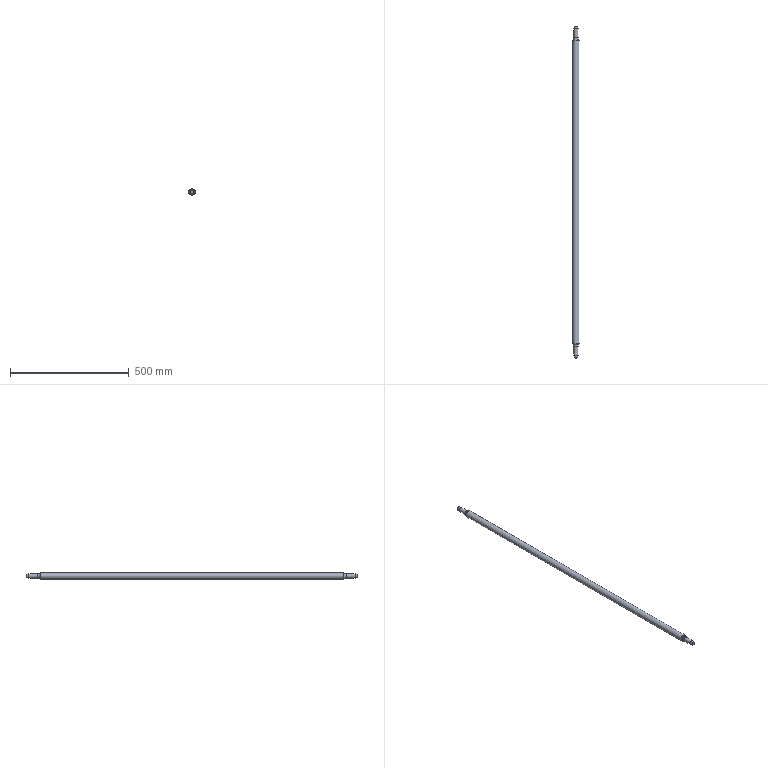Part | NX | features CHAMFER 4, DATUM_CSYS 3, SKETCH 2, Container 1, EXTRACT_BODY 1, EXTRUDE 1, FACE_BLEND 1, Geometry Instance 1, SUBTRACT 1, SWP104 1, SYMBOLIC_THREAD 1 | 1 solid | 31 faces | box 28 x 1395 x 28 mm | volume 817167 mm3 | plane 14 | cylinder 9 | cone 8 | commonest cylinder face diameters 5 x2 16 x2 18 x2 20 x2 28 x1
STEP:
#1=CARTESIAN_POINT('',(2.5,-12.,-7.071));
#2=VERTEX_POINT('',#1);
#3=CARTESIAN_POINT('',(2.5,-12.,-5.));
#4=VERTEX_POINT('',#3);
#5=CARTESIAN_POINT('',(2.5,-12.,-5.));
#6=DIRECTION('',(0.,0.,-1.));
#7=VECTOR('',#6,1000.);
#8=LINE('',#5,#7);
#9=EDGE_CURVE('',#2,#4,#8,.F.);
#10=ORIENTED_EDGE('',*,*,#9,.F.);
#11=CARTESIAN_POINT('',(-2.5,-12.,-7.071));
#12=VERTEX_POINT('',#11);
#13=CARTESIAN_POINT('',(0.,-12.,0.));
#14=DIRECTION('',(0.,1.,0.));
#15=DIRECTION('',(0.,0.,1.));
#16=AXIS2_PLACEMENT_3D('',#13,#14,#15);
#17=CIRCLE('',#16,7.5);
#18=EDGE_CURVE('',#2,#12,#17,.F.);
#19=ORIENTED_EDGE('',*,*,#18,.T.);
#20=CARTESIAN_POINT('',(-2.5,-12.,-5.));
#21=VERTEX_POINT('',#20);
#22=CARTESIAN_POINT('',(-2.5,-12.,-15.));
#23=DIRECTION('',(0.,0.,1.));
#24=VECTOR('',#23,1000.);
#25=LINE('',#22,#24);
#26=EDGE_CURVE('',#21,#12,#25,.F.);
#27=ORIENTED_EDGE('',*,*,#26,.F.);
#28=CARTESIAN_POINT('',(-2.5,-12.,-5.));
#29=DIRECTION('',(1.,0.,0.));
#30=VECTOR('',#29,1000.);
#31=LINE('',#28,#30);
#32=EDGE_CURVE('',#4,#21,#31,.F.);
#33=ORIENTED_EDGE('',*,*,#32,.F.);
#34=EDGE_LOOP('',(#10,#19,#27,#33));
#35=FACE_BOUND('',#34,.T.);
#36=CARTESIAN_POINT('',(0.,-12.,0.));
#37=DIRECTION('',(0.,1.,0.));
#38=DIRECTION('',(0.,0.,1.));
#39=AXIS2_PLACEMENT_3D('',#36,#37,#38);
#40=PLANE('',#39);
#41=ADVANCED_FACE('',(#35),#40,.F.);
#42=CARTESIAN_POINT('',(-2.5,1383.,-7.071));
#43=VERTEX_POINT('',#42);
#44=CARTESIAN_POINT('',(-2.5,1383.,-5.));
#45=VERTEX_POINT('',#44);
#46=CARTESIAN_POINT('',(-2.5,1383.,-15.));
#47=DIRECTION('',(0.,0.,1.));
#48=VECTOR('',#47,1000.);
#49=LINE('',#46,#48);
#50=EDGE_CURVE('',#43,#45,#49,.T.);
#51=ORIENTED_EDGE('',*,*,#50,.F.);
#52=CARTESIAN_POINT('',(2.5,1383.,-7.071));
#53=VERTEX_POINT('',#52);
#54=CARTESIAN_POINT('',(0.,1383.,0.));
#55=DIRECTION('',(0.,1.,0.));
#56=DIRECTION('',(0.,0.,1.));
#57=AXIS2_PLACEMENT_3D('',#54,#55,#56);
#58=CIRCLE('',#57,7.5);
#59=EDGE_CURVE('',#43,#53,#58,.T.);
#60=ORIENTED_EDGE('',*,*,#59,.T.);
#61=CARTESIAN_POINT('',(2.5,1383.,-5.));
#62=VERTEX_POINT('',#61);
#63=CARTESIAN_POINT('',(2.5,1383.,-5.));
#64=DIRECTION('',(0.,0.,-1.));
#65=VECTOR('',#64,1000.);
#66=LINE('',#63,#65);
#67=EDGE_CURVE('',#62,#53,#66,.T.);
#68=ORIENTED_EDGE('',*,*,#67,.F.);
#69=CARTESIAN_POINT('',(-2.5,1383.,-5.));
#70=DIRECTION('',(1.,0.,0.));
#71=VECTOR('',#70,1000.);
#72=LINE('',#69,#71);
#73=EDGE_CURVE('',#45,#62,#72,.T.);
#74=ORIENTED_EDGE('',*,*,#73,.F.);
#75=EDGE_LOOP('',(#51,#60,#68,#74));
#76=FACE_BOUND('',#75,.T.);
#77=CARTESIAN_POINT('',(0.,1383.,0.));
#78=DIRECTION('',(0.,1.,0.));
#79=DIRECTION('',(0.,0.,1.));
#80=AXIS2_PLACEMENT_3D('',#77,#78,#79);
#81=PLANE('',#80);
#82=ADVANCED_FACE('',(#76),#81,.T.);
#83=CARTESIAN_POINT('',(-2.5,-11.5,-7.599));
#84=VERTEX_POINT('',#83);
#85=CARTESIAN_POINT('',(-2.5,-2.5,-7.599));
#86=VERTEX_POINT('',#85);
#87=CARTESIAN_POINT('',(-2.5,0.,-7.599));
#88=DIRECTION('',(0.,1.,0.));
#89=VECTOR('',#88,1000.);
#90=LINE('',#87,#89);
#91=EDGE_CURVE('',#84,#86,#90,.T.);
#92=ORIENTED_EDGE('',*,*,#91,.F.);
#93=CARTESIAN_POINT('',(2.5,-11.5,-7.599));
#94=VERTEX_POINT('',#93);
#95=CARTESIAN_POINT('',(0.,-11.5,0.));
#96=DIRECTION('',(0.,1.,0.));
#97=DIRECTION('',(0.,0.,1.));
#98=AXIS2_PLACEMENT_3D('',#95,#96,#97);
#99=CIRCLE('',#98,8.);
#100=EDGE_CURVE('',#84,#94,#99,.T.);
#101=ORIENTED_EDGE('',*,*,#100,.T.);
#102=CARTESIAN_POINT('',(2.5,-2.5,-7.599));
#103=VERTEX_POINT('',#102);
#104=CARTESIAN_POINT('',(2.5,0.,-7.599));
#105=DIRECTION('',(0.,1.,0.));
#106=VECTOR('',#105,1000.);
#107=LINE('',#104,#106);
#108=EDGE_CURVE('',#103,#94,#107,.F.);
#109=ORIENTED_EDGE('',*,*,#108,.F.);
#110=CARTESIAN_POINT('',(0.,0.,-8.));
#111=VERTEX_POINT('',#110);
#112=CARTESIAN_POINT('',(0.,0.,-8.));
#113=CARTESIAN_POINT('',(0.6564,0.,-8.));
#114=CARTESIAN_POINT('',(1.958,-0.5475,-7.805));
#115=CARTESIAN_POINT('',(2.5,-1.835,-7.599));
#116=CARTESIAN_POINT('',(2.5,-2.5,-7.599));
#117=B_SPLINE_CURVE_WITH_KNOTS('',3,(#112,#113,#114,#115,#116),.UNSPECIFIED.,.F.,.F.,(4,1,4),(0.003934,0.005898,0.007863),.UNSPECIFIED.);
#118=EDGE_CURVE('',#111,#103,#117,.T.);
#119=ORIENTED_EDGE('',*,*,#118,.F.);
#120=CARTESIAN_POINT('',(0.,0.,0.));
#121=DIRECTION('',(0.,1.,0.));
#122=DIRECTION('',(0.,0.,1.));
#123=AXIS2_PLACEMENT_3D('',#120,#121,#122);
#124=CIRCLE('',#123,8.);
#125=EDGE_CURVE('',#111,#111,#124,.T.);
#126=ORIENTED_EDGE('',*,*,#125,.F.);
#127=CARTESIAN_POINT('',(-2.5,-2.5,-7.599));
#128=CARTESIAN_POINT('',(-2.5,-1.835,-7.599));
#129=CARTESIAN_POINT('',(-1.955,-0.5457,-7.805));
#130=CARTESIAN_POINT('',(-0.6572,0.,-8.));
#131=CARTESIAN_POINT('',(0.,0.,-8.));
#132=B_SPLINE_CURVE_WITH_KNOTS('',3,(#127,#128,#129,#130,#131),.UNSPECIFIED.,.F.,.F.,(4,1,4),(0.,0.001967,0.003934),.UNSPECIFIED.);
#133=EDGE_CURVE('',#86,#111,#132,.T.);
#134=ORIENTED_EDGE('',*,*,#133,.F.);
#135=EDGE_LOOP('',(#92,#101,#109,#119,#126,#134));
#136=FACE_BOUND('',#135,.T.);
#137=CARTESIAN_POINT('',(0.,0.,0.));
#138=DIRECTION('',(0.,1.,0.));
#139=DIRECTION('',(0.,0.,1.));
#140=AXIS2_PLACEMENT_3D('',#137,#138,#139);
#141=CYLINDRICAL_SURFACE('',#140,8.);
#142=ADVANCED_FACE('',(#136),#141,.T.);
#143=CARTESIAN_POINT('',(0.,0.,-8.5));
#144=VERTEX_POINT('',#143);
#145=CARTESIAN_POINT('',(0.,0.,0.));
#146=DIRECTION('',(0.,-1.,0.));
#147=DIRECTION('',(0.,0.,-1.));
#148=AXIS2_PLACEMENT_3D('',#145,#146,#147);
#149=CIRCLE('',#148,8.5);
#150=EDGE_CURVE('',#144,#144,#149,.T.);
#151=ORIENTED_EDGE('',*,*,#150,.T.);
#152=EDGE_LOOP('',(#151));
#153=FACE_BOUND('',#152,.T.);
#154=ORIENTED_EDGE('',*,*,#125,.T.);
#155=EDGE_LOOP('',(#154));
#156=FACE_BOUND('',#155,.T.);
#157=CARTESIAN_POINT('',(0.,0.,9.));
#158=DIRECTION('',(0.,-1.,0.));
#159=DIRECTION('',(0.,0.,-1.));
#160=AXIS2_PLACEMENT_3D('',#157,#158,#159);
#161=PLANE('',#160);
#162=ADVANCED_FACE('',(#153,#156),#161,.T.);
#163=CARTESIAN_POINT('',(0.,0.5,-9.));
#164=VERTEX_POINT('',#163);
#165=CARTESIAN_POINT('',(0.,0.5,0.));
#166=DIRECTION('',(0.,-1.,0.));
#167=DIRECTION('',(0.,0.,-1.));
#168=AXIS2_PLACEMENT_3D('',#165,#166,#167);
#169=CIRCLE('',#168,9.);
#170=EDGE_CURVE('',#164,#164,#169,.F.);
#171=ORIENTED_EDGE('',*,*,#170,.T.);
#172=EDGE_LOOP('',(#171));
#173=FACE_BOUND('',#172,.T.);
#174=CARTESIAN_POINT('',(0.,35.,9.));
#175=VERTEX_POINT('',#174);
#176=CARTESIAN_POINT('',(0.,35.,0.));
#177=DIRECTION('',(0.,1.,0.));
#178=DIRECTION('',(0.,0.,1.));
#179=AXIS2_PLACEMENT_3D('',#176,#177,#178);
#180=CIRCLE('',#179,9.);
#181=EDGE_CURVE('',#175,#175,#180,.T.);
#182=ORIENTED_EDGE('',*,*,#181,.F.);
#183=EDGE_LOOP('',(#182));
#184=FACE_BOUND('',#183,.T.);
#185=CARTESIAN_POINT('',(0.,0.,0.));
#186=DIRECTION('',(0.,1.,0.));
#187=DIRECTION('',(0.,0.,1.));
#188=AXIS2_PLACEMENT_3D('',#185,#186,#187);
#189=CYLINDRICAL_SURFACE('',#188,9.);
#190=ADVANCED_FACE('',(#173,#184),#189,.T.);
#191=CARTESIAN_POINT('',(0.,35.,-9.5));
#192=VERTEX_POINT('',#191);
#193=CARTESIAN_POINT('',(0.,35.,0.));
#194=DIRECTION('',(0.,-1.,0.));
#195=DIRECTION('',(0.,0.,-1.));
#196=AXIS2_PLACEMENT_3D('',#193,#194,#195);
#197=CIRCLE('',#196,9.5);
#198=EDGE_CURVE('',#192,#192,#197,.T.);
#199=ORIENTED_EDGE('',*,*,#198,.T.);
#200=EDGE_LOOP('',(#199));
#201=FACE_BOUND('',#200,.T.);
#202=ORIENTED_EDGE('',*,*,#181,.T.);
#203=EDGE_LOOP('',(#202));
#204=FACE_BOUND('',#203,.T.);
#205=CARTESIAN_POINT('',(0.,35.,10.));
#206=DIRECTION('',(0.,-1.,0.));
#207=DIRECTION('',(0.,0.,-1.));
#208=AXIS2_PLACEMENT_3D('',#205,#206,#207);
#209=PLANE('',#208);
#210=ADVANCED_FACE('',(#201,#204),#209,.T.);
#211=CARTESIAN_POINT('',(0.,35.5,-10.));
#212=VERTEX_POINT('',#211);
#213=CARTESIAN_POINT('',(0.,35.5,0.));
#214=DIRECTION('',(0.,-1.,0.));
#215=DIRECTION('',(0.,0.,-1.));
#216=AXIS2_PLACEMENT_3D('',#213,#214,#215);
#217=CIRCLE('',#216,10.);
#218=EDGE_CURVE('',#212,#212,#217,.F.);
#219=ORIENTED_EDGE('',*,*,#218,.T.);
#220=EDGE_LOOP('',(#219));
#221=FACE_BOUND('',#220,.T.);
#222=CARTESIAN_POINT('',(0.,44.,10.));
#223=VERTEX_POINT('',#222);
#224=CARTESIAN_POINT('',(0.,44.,0.));
#225=DIRECTION('',(0.,1.,0.));
#226=DIRECTION('',(0.,0.,1.));
#227=AXIS2_PLACEMENT_3D('',#224,#225,#226);
#228=CIRCLE('',#227,10.);
#229=EDGE_CURVE('',#223,#223,#228,.T.);
#230=ORIENTED_EDGE('',*,*,#229,.F.);
#231=EDGE_LOOP('',(#230));
#232=FACE_BOUND('',#231,.T.);
#233=CARTESIAN_POINT('',(0.,0.,0.));
#234=DIRECTION('',(0.,1.,0.));
#235=DIRECTION('',(0.,0.,1.));
#236=AXIS2_PLACEMENT_3D('',#233,#234,#235);
#237=CYLINDRICAL_SURFACE('',#236,10.);
#238=ADVANCED_FACE('',(#221,#232),#237,.T.);
#239=CARTESIAN_POINT('',(0.,44.,-11.));
#240=VERTEX_POINT('',#239);
#241=CARTESIAN_POINT('',(0.,44.,0.));
#242=DIRECTION('',(0.,-1.,0.));
#243=DIRECTION('',(0.,0.,-1.));
#244=AXIS2_PLACEMENT_3D('',#241,#242,#243);
#245=CIRCLE('',#244,11.);
#246=EDGE_CURVE('',#240,#240,#245,.T.);
#247=ORIENTED_EDGE('',*,*,#246,.T.);
#248=EDGE_LOOP('',(#247));
#249=FACE_BOUND('',#248,.T.);
#250=ORIENTED_EDGE('',*,*,#229,.T.);
#251=EDGE_LOOP('',(#250));
#252=FACE_BOUND('',#251,.T.);
#253=CARTESIAN_POINT('',(0.,44.,14.));
#254=DIRECTION('',(0.,-1.,0.));
#255=DIRECTION('',(0.,0.,-1.));
#256=AXIS2_PLACEMENT_3D('',#253,#254,#255);
#257=PLANE('',#256);
#258=ADVANCED_FACE('',(#249,#252),#257,.T.);
#259=CARTESIAN_POINT('',(0.,1324.,14.));
#260=VERTEX_POINT('',#259);
#261=CARTESIAN_POINT('',(0.,1324.,0.));
#262=DIRECTION('',(0.,1.,0.));
#263=DIRECTION('',(0.,0.,1.));
#264=AXIS2_PLACEMENT_3D('',#261,#262,#263);
#265=CIRCLE('',#264,14.);
#266=EDGE_CURVE('',#260,#260,#265,.F.);
#267=ORIENTED_EDGE('',*,*,#266,.T.);
#268=EDGE_LOOP('',(#267));
#269=FACE_BOUND('',#268,.T.);
#270=CARTESIAN_POINT('',(0.,47.,-14.));
#271=VERTEX_POINT('',#270);
#272=CARTESIAN_POINT('',(0.,47.,0.));
#273=DIRECTION('',(0.,-1.,0.));
#274=DIRECTION('',(0.,0.,-1.));
#275=AXIS2_PLACEMENT_3D('',#272,#273,#274);
#276=CIRCLE('',#275,14.);
#277=EDGE_CURVE('',#271,#271,#276,.F.);
#278=ORIENTED_EDGE('',*,*,#277,.T.);
#279=EDGE_LOOP('',(#278));
#280=FACE_BOUND('',#279,.T.);
#281=CARTESIAN_POINT('',(0.,0.,0.));
#282=DIRECTION('',(0.,1.,0.));
#283=DIRECTION('',(0.,0.,1.));
#284=AXIS2_PLACEMENT_3D('',#281,#282,#283);
#285=CYLINDRICAL_SURFACE('',#284,14.);
#286=ADVANCED_FACE('',(#269,#280),#285,.T.);
#287=CARTESIAN_POINT('',(0.,1327.,11.));
#288=VERTEX_POINT('',#287);
#289=CARTESIAN_POINT('',(0.,1327.,0.));
#290=DIRECTION('',(0.,1.,0.));
#291=DIRECTION('',(0.,0.,1.));
#292=AXIS2_PLACEMENT_3D('',#289,#290,#291);
#293=CIRCLE('',#292,11.);
#294=EDGE_CURVE('',#288,#288,#293,.T.);
#295=ORIENTED_EDGE('',*,*,#294,.T.);
#296=EDGE_LOOP('',(#295));
#297=FACE_BOUND('',#296,.T.);
#298=CARTESIAN_POINT('',(0.,1327.,10.));
#299=VERTEX_POINT('',#298);
#300=CARTESIAN_POINT('',(0.,1327.,0.));
#301=DIRECTION('',(0.,1.,0.));
#302=DIRECTION('',(0.,0.,1.));
#303=AXIS2_PLACEMENT_3D('',#300,#301,#302);
#304=CIRCLE('',#303,10.);
#305=EDGE_CURVE('',#299,#299,#304,.T.);
#306=ORIENTED_EDGE('',*,*,#305,.F.);
#307=EDGE_LOOP('',(#306));
#308=FACE_BOUND('',#307,.T.);
#309=CARTESIAN_POINT('',(0.,1327.,10.));
#310=DIRECTION('',(0.,1.,0.));
#311=DIRECTION('',(0.,0.,1.));
#312=AXIS2_PLACEMENT_3D('',#309,#310,#311);
#313=PLANE('',#312);
#314=ADVANCED_FACE('',(#297,#308),#313,.T.);
#315=CARTESIAN_POINT('',(0.,1335.5,10.));
#316=VERTEX_POINT('',#315);
#317=CARTESIAN_POINT('',(0.,1335.5,0.));
#318=DIRECTION('',(0.,1.,0.));
#319=DIRECTION('',(0.,0.,1.));
#320=AXIS2_PLACEMENT_3D('',#317,#318,#319);
#321=CIRCLE('',#320,10.);
#322=EDGE_CURVE('',#316,#316,#321,.F.);
#323=ORIENTED_EDGE('',*,*,#322,.T.);
#324=EDGE_LOOP('',(#323));
#325=FACE_BOUND('',#324,.T.);
#326=ORIENTED_EDGE('',*,*,#305,.T.);
#327=EDGE_LOOP('',(#326));
#328=FACE_BOUND('',#327,.T.);
#329=CARTESIAN_POINT('',(0.,0.,0.));
#330=DIRECTION('',(0.,1.,0.));
#331=DIRECTION('',(0.,0.,1.));
#332=AXIS2_PLACEMENT_3D('',#329,#330,#331);
#333=CYLINDRICAL_SURFACE('',#332,10.);
#334=ADVANCED_FACE('',(#325,#328),#333,.T.);
#335=CARTESIAN_POINT('',(0.,1336.,9.5));
#336=VERTEX_POINT('',#335);
#337=CARTESIAN_POINT('',(0.,1336.,0.));
#338=DIRECTION('',(0.,1.,0.));
#339=DIRECTION('',(0.,0.,1.));
#340=AXIS2_PLACEMENT_3D('',#337,#338,#339);
#341=CIRCLE('',#340,9.5);
#342=EDGE_CURVE('',#336,#336,#341,.T.);
#343=ORIENTED_EDGE('',*,*,#342,.T.);
#344=EDGE_LOOP('',(#343));
#345=FACE_BOUND('',#344,.T.);
#346=CARTESIAN_POINT('',(0.,1336.,9.));
#347=VERTEX_POINT('',#346);
#348=CARTESIAN_POINT('',(0.,1336.,0.));
#349=DIRECTION('',(0.,1.,0.));
#350=DIRECTION('',(0.,0.,1.));
#351=AXIS2_PLACEMENT_3D('',#348,#349,#350);
#352=CIRCLE('',#351,9.);
#353=EDGE_CURVE('',#347,#347,#352,.T.);
#354=ORIENTED_EDGE('',*,*,#353,.F.);
#355=EDGE_LOOP('',(#354));
#356=FACE_BOUND('',#355,.T.);
#357=CARTESIAN_POINT('',(0.,1336.,9.));
#358=DIRECTION('',(0.,1.,0.));
#359=DIRECTION('',(0.,0.,1.));
#360=AXIS2_PLACEMENT_3D('',#357,#358,#359);
#361=PLANE('',#360);
#362=ADVANCED_FACE('',(#345,#356),#361,.T.);
#363=CARTESIAN_POINT('',(0.,1370.5,9.));
#364=VERTEX_POINT('',#363);
#365=CARTESIAN_POINT('',(0.,1370.5,0.));
#366=DIRECTION('',(0.,1.,0.));
#367=DIRECTION('',(0.,0.,1.));
#368=AXIS2_PLACEMENT_3D('',#365,#366,#367);
#369=CIRCLE('',#368,9.);
#370=EDGE_CURVE('',#364,#364,#369,.F.);
#371=ORIENTED_EDGE('',*,*,#370,.T.);
#372=EDGE_LOOP('',(#371));
#373=FACE_BOUND('',#372,.T.);
#374=ORIENTED_EDGE('',*,*,#353,.T.);
#375=EDGE_LOOP('',(#374));
#376=FACE_BOUND('',#375,.T.);
#377=CARTESIAN_POINT('',(0.,0.,0.));
#378=DIRECTION('',(0.,1.,0.));
#379=DIRECTION('',(0.,0.,1.));
#380=AXIS2_PLACEMENT_3D('',#377,#378,#379);
#381=CYLINDRICAL_SURFACE('',#380,9.);
#382=ADVANCED_FACE('',(#373,#376),#381,.T.);
#383=CARTESIAN_POINT('',(0.,1371.,8.5));
#384=VERTEX_POINT('',#383);
#385=CARTESIAN_POINT('',(0.,1371.,0.));
#386=DIRECTION('',(0.,1.,0.));
#387=DIRECTION('',(0.,0.,1.));
#388=AXIS2_PLACEMENT_3D('',#385,#386,#387);
#389=CIRCLE('',#388,8.5);
#390=EDGE_CURVE('',#384,#384,#389,.T.);
#391=ORIENTED_EDGE('',*,*,#390,.T.);
#392=EDGE_LOOP('',(#391));
#393=FACE_BOUND('',#392,.T.);
#394=CARTESIAN_POINT('',(0.,1371.,-8.));
#395=VERTEX_POINT('',#394);
#396=CARTESIAN_POINT('',(0.,1371.,0.));
#397=DIRECTION('',(0.,1.,0.));
#398=DIRECTION('',(0.,0.,1.));
#399=AXIS2_PLACEMENT_3D('',#396,#397,#398);
#400=CIRCLE('',#399,8.);
#401=EDGE_CURVE('',#395,#395,#400,.T.);
#402=ORIENTED_EDGE('',*,*,#401,.F.);
#403=EDGE_LOOP('',(#402));
#404=FACE_BOUND('',#403,.T.);
#405=CARTESIAN_POINT('',(0.,1371.,8.));
#406=DIRECTION('',(0.,1.,0.));
#407=DIRECTION('',(0.,0.,1.));
#408=AXIS2_PLACEMENT_3D('',#405,#406,#407);
#409=PLANE('',#408);
#410=ADVANCED_FACE('',(#393,#404),#409,.T.);
#411=CARTESIAN_POINT('',(2.5,1382.5,-7.599));
#412=VERTEX_POINT('',#411);
#413=CARTESIAN_POINT('',(2.5,1373.5,-7.599));
#414=VERTEX_POINT('',#413);
#415=CARTESIAN_POINT('',(2.5,0.,-7.599));
#416=DIRECTION('',(0.,1.,0.));
#417=VECTOR('',#416,1000.);
#418=LINE('',#415,#417);
#419=EDGE_CURVE('',#412,#414,#418,.F.);
#420=ORIENTED_EDGE('',*,*,#419,.F.);
#421=CARTESIAN_POINT('',(-2.5,1382.5,-7.599));
#422=VERTEX_POINT('',#421);
#423=CARTESIAN_POINT('',(0.,1382.5,0.));
#424=DIRECTION('',(0.,1.,0.));
#425=DIRECTION('',(0.,0.,1.));
#426=AXIS2_PLACEMENT_3D('',#423,#424,#425);
#427=CIRCLE('',#426,8.);
#428=EDGE_CURVE('',#412,#422,#427,.F.);
#429=ORIENTED_EDGE('',*,*,#428,.T.);
#430=CARTESIAN_POINT('',(-2.5,1373.5,-7.599));
#431=VERTEX_POINT('',#430);
#432=CARTESIAN_POINT('',(-2.5,0.,-7.599));
#433=DIRECTION('',(0.,1.,0.));
#434=VECTOR('',#433,1000.);
#435=LINE('',#432,#434);
#436=EDGE_CURVE('',#431,#422,#435,.T.);
#437=ORIENTED_EDGE('',*,*,#436,.F.);
#438=CARTESIAN_POINT('',(0.,1371.,-8.));
#439=CARTESIAN_POINT('',(-0.6564,1371.,-8.));
#440=CARTESIAN_POINT('',(-1.958,1371.548,-7.805));
#441=CARTESIAN_POINT('',(-2.5,1372.835,-7.599));
#442=CARTESIAN_POINT('',(-2.5,1373.5,-7.599));
#443=B_SPLINE_CURVE_WITH_KNOTS('',3,(#438,#439,#440,#441,#442),.UNSPECIFIED.,.F.,.F.,(4,1,4),(0.003934,0.005898,0.007863),.UNSPECIFIED.);
#444=EDGE_CURVE('',#395,#431,#443,.T.);
#445=ORIENTED_EDGE('',*,*,#444,.F.);
#446=ORIENTED_EDGE('',*,*,#401,.T.);
#447=CARTESIAN_POINT('',(2.5,1373.5,-7.599));
#448=CARTESIAN_POINT('',(2.5,1372.835,-7.599));
#449=CARTESIAN_POINT('',(1.955,1371.546,-7.805));
#450=CARTESIAN_POINT('',(0.6572,1371.,-8.));
#451=CARTESIAN_POINT('',(0.,1371.,-8.));
#452=B_SPLINE_CURVE_WITH_KNOTS('',3,(#447,#448,#449,#450,#451),.UNSPECIFIED.,.F.,.F.,(4,1,4),(0.,0.001967,0.003934),.UNSPECIFIED.);
#453=EDGE_CURVE('',#414,#395,#452,.T.);
#454=ORIENTED_EDGE('',*,*,#453,.F.);
#455=EDGE_LOOP('',(#420,#429,#437,#445,#446,#454));
#456=FACE_BOUND('',#455,.T.);
#457=CARTESIAN_POINT('',(0.,0.,0.));
#458=DIRECTION('',(0.,1.,0.));
#459=DIRECTION('',(0.,0.,1.));
#460=AXIS2_PLACEMENT_3D('',#457,#458,#459);
#461=CYLINDRICAL_SURFACE('',#460,8.);
#462=ADVANCED_FACE('',(#456),#461,.T.);
#463=ORIENTED_EDGE('',*,*,#453,.T.);
#464=ORIENTED_EDGE('',*,*,#444,.T.);
#465=CARTESIAN_POINT('',(-2.5,1373.5,-5.));
#466=VERTEX_POINT('',#465);
#467=CARTESIAN_POINT('',(-2.5,1373.5,-5.));
#468=DIRECTION('',(0.,0.,1.));
#469=VECTOR('',#468,1000.);
#470=LINE('',#467,#469);
#471=EDGE_CURVE('',#466,#431,#470,.F.);
#472=ORIENTED_EDGE('',*,*,#471,.F.);
#473=CARTESIAN_POINT('',(2.5,1373.5,-5.));
#474=VERTEX_POINT('',#473);
#475=CARTESIAN_POINT('',(0.,1373.5,-5.));
#476=DIRECTION('',(0.,0.,1.));
#477=DIRECTION('',(1.,0.,0.));
#478=AXIS2_PLACEMENT_3D('',#475,#476,#477);
#479=CIRCLE('',#478,2.5);
#480=EDGE_CURVE('',#474,#466,#479,.F.);
#481=ORIENTED_EDGE('',*,*,#480,.F.);
#482=CARTESIAN_POINT('',(2.5,1373.5,-5.));
#483=DIRECTION('',(0.,0.,1.));
#484=VECTOR('',#483,1000.);
#485=LINE('',#482,#484);
#486=EDGE_CURVE('',#414,#474,#485,.T.);
#487=ORIENTED_EDGE('',*,*,#486,.F.);
#488=EDGE_LOOP('',(#463,#464,#472,#481,#487));
#489=FACE_BOUND('',#488,.T.);
#490=CARTESIAN_POINT('',(0.,1373.5,-5.));
#491=DIRECTION('',(0.,0.,-1.));
#492=DIRECTION('',(-1.,0.,0.));
#493=AXIS2_PLACEMENT_3D('',#490,#491,#492);
#494=CYLINDRICAL_SURFACE('',#493,2.5);
#495=ADVANCED_FACE('',(#489),#494,.F.);
#496=ORIENTED_EDGE('',*,*,#67,.T.);
#497=CARTESIAN_POINT('',(2.5,1383.,-7.071));
#498=CARTESIAN_POINT('',(2.5,1382.834,-7.247));
#499=CARTESIAN_POINT('',(2.5,1382.667,-7.424));
#500=CARTESIAN_POINT('',(2.5,1382.5,-7.599));
#501=B_SPLINE_CURVE_WITH_KNOTS('',3,(#497,#498,#499,#500),.UNSPECIFIED.,.F.,.F.,(4,4),(0.,0.0007274),.UNSPECIFIED.);
#502=EDGE_CURVE('',#53,#412,#501,.T.);
#503=ORIENTED_EDGE('',*,*,#502,.T.);
#504=ORIENTED_EDGE('',*,*,#419,.T.);
#505=ORIENTED_EDGE('',*,*,#486,.T.);
#506=CARTESIAN_POINT('',(2.5,1264.2,-5.));
#507=DIRECTION('',(0.,1.,0.));
#508=VECTOR('',#507,1000.);
#509=LINE('',#506,#508);
#510=EDGE_CURVE('',#62,#474,#509,.F.);
#511=ORIENTED_EDGE('',*,*,#510,.F.);
#512=EDGE_LOOP('',(#496,#503,#504,#505,#511));
#513=FACE_BOUND('',#512,.T.);
#514=CARTESIAN_POINT('',(2.5,1264.2,-5.));
#515=DIRECTION('',(1.,0.,0.));
#516=DIRECTION('',(0.,0.,-1.));
#517=AXIS2_PLACEMENT_3D('',#514,#515,#516);
#518=PLANE('',#517);
#519=ADVANCED_FACE('',(#513),#518,.F.);
#520=CARTESIAN_POINT('',(-2.5,1264.2,-5.));
#521=DIRECTION('',(0.,1.,0.));
#522=VECTOR('',#521,1000.);
#523=LINE('',#520,#522);
#524=EDGE_CURVE('',#45,#466,#523,.F.);
#525=ORIENTED_EDGE('',*,*,#524,.F.);
#526=ORIENTED_EDGE('',*,*,#73,.T.);
#527=ORIENTED_EDGE('',*,*,#510,.T.);
#528=ORIENTED_EDGE('',*,*,#480,.T.);
#529=EDGE_LOOP('',(#525,#526,#527,#528));
#530=FACE_BOUND('',#529,.T.);
#531=CARTESIAN_POINT('',(-2.5,1264.2,-5.));
#532=DIRECTION('',(0.,0.,1.));
#533=DIRECTION('',(1.,0.,0.));
#534=AXIS2_PLACEMENT_3D('',#531,#532,#533);
#535=PLANE('',#534);
#536=ADVANCED_FACE('',(#530),#535,.F.);
#537=ORIENTED_EDGE('',*,*,#436,.T.);
#538=CARTESIAN_POINT('',(-2.5,1382.5,-7.599));
#539=CARTESIAN_POINT('',(-2.5,1382.667,-7.424));
#540=CARTESIAN_POINT('',(-2.5,1382.834,-7.247));
#541=CARTESIAN_POINT('',(-2.5,1383.,-7.071));
#542=B_SPLINE_CURVE_WITH_KNOTS('',3,(#538,#539,#540,#541),.UNSPECIFIED.,.F.,.F.,(4,4),(0.,0.0007274),.UNSPECIFIED.);
#543=EDGE_CURVE('',#422,#43,#542,.T.);
#544=ORIENTED_EDGE('',*,*,#543,.T.);
#545=ORIENTED_EDGE('',*,*,#50,.T.);
#546=ORIENTED_EDGE('',*,*,#524,.T.);
#547=ORIENTED_EDGE('',*,*,#471,.T.);
#548=EDGE_LOOP('',(#537,#544,#545,#546,#547));
#549=FACE_BOUND('',#548,.T.);
#550=CARTESIAN_POINT('',(-2.5,1264.2,-15.));
#551=DIRECTION('',(-1.,0.,0.));
#552=DIRECTION('',(0.,0.,1.));
#553=AXIS2_PLACEMENT_3D('',#550,#551,#552);
#554=PLANE('',#553);
#555=ADVANCED_FACE('',(#549),#554,.F.);
#556=ORIENTED_EDGE('',*,*,#133,.T.);
#557=ORIENTED_EDGE('',*,*,#118,.T.);
#558=CARTESIAN_POINT('',(2.5,-2.5,-5.));
#559=VERTEX_POINT('',#558);
#560=CARTESIAN_POINT('',(2.5,-2.5,-5.));
#561=DIRECTION('',(0.,0.,1.));
#562=VECTOR('',#561,1000.);
#563=LINE('',#560,#562);
#564=EDGE_CURVE('',#559,#103,#563,.F.);
#565=ORIENTED_EDGE('',*,*,#564,.F.);
#566=CARTESIAN_POINT('',(-2.5,-2.5,-5.));
#567=VERTEX_POINT('',#566);
#568=CARTESIAN_POINT('',(0.,-2.5,-5.));
#569=DIRECTION('',(0.,0.,-1.));
#570=DIRECTION('',(1.,0.,0.));
#571=AXIS2_PLACEMENT_3D('',#568,#569,#570);
#572=CIRCLE('',#571,2.5);
#573=EDGE_CURVE('',#567,#559,#572,.T.);
#574=ORIENTED_EDGE('',*,*,#573,.F.);
#575=CARTESIAN_POINT('',(-2.5,-2.5,-5.));
#576=DIRECTION('',(0.,0.,1.));
#577=VECTOR('',#576,1000.);
#578=LINE('',#575,#577);
#579=EDGE_CURVE('',#86,#567,#578,.T.);
#580=ORIENTED_EDGE('',*,*,#579,.F.);
#581=EDGE_LOOP('',(#556,#557,#565,#574,#580));
#582=FACE_BOUND('',#581,.T.);
#583=CARTESIAN_POINT('',(0.,-2.5,-5.));
#584=DIRECTION('',(0.,0.,-1.));
#585=DIRECTION('',(-1.,0.,0.));
#586=AXIS2_PLACEMENT_3D('',#583,#584,#585);
#587=CYLINDRICAL_SURFACE('',#586,2.5);
#588=ADVANCED_FACE('',(#582),#587,.F.);
#589=ORIENTED_EDGE('',*,*,#26,.T.);
#590=CARTESIAN_POINT('',(-2.5,-12.,-7.071));
#591=CARTESIAN_POINT('',(-2.5,-11.834,-7.247));
#592=CARTESIAN_POINT('',(-2.5,-11.667,-7.424));
#593=CARTESIAN_POINT('',(-2.5,-11.5,-7.599));
#594=B_SPLINE_CURVE_WITH_KNOTS('',3,(#590,#591,#592,#593),.UNSPECIFIED.,.F.,.F.,(4,4),(0.,0.0007274),.UNSPECIFIED.);
#595=EDGE_CURVE('',#12,#84,#594,.T.);
#596=ORIENTED_EDGE('',*,*,#595,.T.);
#597=ORIENTED_EDGE('',*,*,#91,.T.);
#598=ORIENTED_EDGE('',*,*,#579,.T.);
#599=CARTESIAN_POINT('',(-2.5,106.8,-5.));
#600=DIRECTION('',(0.,-1.,0.));
#601=VECTOR('',#600,1000.);
#602=LINE('',#599,#601);
#603=EDGE_CURVE('',#567,#21,#602,.T.);
#604=ORIENTED_EDGE('',*,*,#603,.T.);
#605=EDGE_LOOP('',(#589,#596,#597,#598,#604));
#606=FACE_BOUND('',#605,.T.);
#607=CARTESIAN_POINT('',(-2.5,106.8,-15.));
#608=DIRECTION('',(-1.,0.,0.));
#609=DIRECTION('',(0.,0.,1.));
#610=AXIS2_PLACEMENT_3D('',#607,#608,#609);
#611=PLANE('',#610);
#612=ADVANCED_FACE('',(#606),#611,.F.);
#613=ORIENTED_EDGE('',*,*,#603,.F.);
#614=ORIENTED_EDGE('',*,*,#573,.T.);
#615=CARTESIAN_POINT('',(2.5,106.8,-5.));
#616=DIRECTION('',(0.,-1.,0.));
#617=VECTOR('',#616,1000.);
#618=LINE('',#615,#617);
#619=EDGE_CURVE('',#559,#4,#618,.T.);
#620=ORIENTED_EDGE('',*,*,#619,.T.);
#621=ORIENTED_EDGE('',*,*,#32,.T.);
#622=EDGE_LOOP('',(#613,#614,#620,#621));
#623=FACE_BOUND('',#622,.T.);
#624=CARTESIAN_POINT('',(-2.5,106.8,-5.));
#625=DIRECTION('',(0.,0.,1.));
#626=DIRECTION('',(1.,0.,0.));
#627=AXIS2_PLACEMENT_3D('',#624,#625,#626);
#628=PLANE('',#627);
#629=ADVANCED_FACE('',(#623),#628,.F.);
#630=ORIENTED_EDGE('',*,*,#108,.T.);
#631=CARTESIAN_POINT('',(2.5,-11.5,-7.599));
#632=CARTESIAN_POINT('',(2.5,-11.667,-7.424));
#633=CARTESIAN_POINT('',(2.5,-11.834,-7.247));
#634=CARTESIAN_POINT('',(2.5,-12.,-7.071));
#635=B_SPLINE_CURVE_WITH_KNOTS('',3,(#631,#632,#633,#634),.UNSPECIFIED.,.F.,.F.,(4,4),(0.,0.0007274),.UNSPECIFIED.);
#636=EDGE_CURVE('',#94,#2,#635,.T.);
#637=ORIENTED_EDGE('',*,*,#636,.T.);
#638=ORIENTED_EDGE('',*,*,#9,.T.);
#639=ORIENTED_EDGE('',*,*,#619,.F.);
#640=ORIENTED_EDGE('',*,*,#564,.T.);
#641=EDGE_LOOP('',(#630,#637,#638,#639,#640));
#642=FACE_BOUND('',#641,.T.);
#643=CARTESIAN_POINT('',(2.5,106.8,-5.));
#644=DIRECTION('',(1.,0.,0.));
#645=DIRECTION('',(0.,0.,-1.));
#646=AXIS2_PLACEMENT_3D('',#643,#644,#645);
#647=PLANE('',#646);
#648=ADVANCED_FACE('',(#642),#647,.F.);
#649=ORIENTED_EDGE('',*,*,#266,.F.);
#650=EDGE_LOOP('',(#649));
#651=FACE_BOUND('',#650,.T.);
#652=ORIENTED_EDGE('',*,*,#294,.F.);
#653=EDGE_LOOP('',(#652));
#654=FACE_BOUND('',#653,.T.);
#655=CARTESIAN_POINT('',(0.,1327.,0.));
#656=DIRECTION('',(0.,-1.,0.));
#657=DIRECTION('',(0.,0.,-1.));
#658=AXIS2_PLACEMENT_3D('',#655,#656,#657);
#659=CONICAL_SURFACE('',#658,11.,0.7854);
#660=ADVANCED_FACE('',(#651,#654),#659,.T.);
#661=ORIENTED_EDGE('',*,*,#246,.F.);
#662=EDGE_LOOP('',(#661));
#663=FACE_BOUND('',#662,.T.);
#664=ORIENTED_EDGE('',*,*,#277,.F.);
#665=EDGE_LOOP('',(#664));
#666=FACE_BOUND('',#665,.T.);
#667=CARTESIAN_POINT('',(0.,47.,0.));
#668=DIRECTION('',(0.,1.,0.));
#669=DIRECTION('',(0.,0.,1.));
#670=AXIS2_PLACEMENT_3D('',#667,#668,#669);
#671=CONICAL_SURFACE('',#670,14.,0.7854);
#672=ADVANCED_FACE('',(#663,#666),#671,.T.);
#673=ORIENTED_EDGE('',*,*,#150,.F.);
#674=EDGE_LOOP('',(#673));
#675=FACE_BOUND('',#674,.T.);
#676=ORIENTED_EDGE('',*,*,#170,.F.);
#677=EDGE_LOOP('',(#676));
#678=FACE_BOUND('',#677,.T.);
#679=CARTESIAN_POINT('',(0.,0.5,0.));
#680=DIRECTION('',(0.,1.,0.));
#681=DIRECTION('',(0.,0.,1.));
#682=AXIS2_PLACEMENT_3D('',#679,#680,#681);
#683=CONICAL_SURFACE('',#682,9.,0.7854);
#684=ADVANCED_FACE('',(#675,#678),#683,.T.);
#685=ORIENTED_EDGE('',*,*,#595,.F.);
#686=ORIENTED_EDGE('',*,*,#18,.F.);
#687=ORIENTED_EDGE('',*,*,#636,.F.);
#688=ORIENTED_EDGE('',*,*,#100,.F.);
#689=EDGE_LOOP('',(#685,#686,#687,#688));
#690=FACE_BOUND('',#689,.T.);
#691=CARTESIAN_POINT('',(0.,-11.5,0.));
#692=DIRECTION('',(0.,1.,0.));
#693=DIRECTION('',(0.,0.,1.));
#694=AXIS2_PLACEMENT_3D('',#691,#692,#693);
#695=CONICAL_SURFACE('',#694,8.,0.7854);
#696=ADVANCED_FACE('',(#690),#695,.T.);
#697=ORIENTED_EDGE('',*,*,#198,.F.);
#698=EDGE_LOOP('',(#697));
#699=FACE_BOUND('',#698,.T.);
#700=ORIENTED_EDGE('',*,*,#218,.F.);
#701=EDGE_LOOP('',(#700));
#702=FACE_BOUND('',#701,.T.);
#703=CARTESIAN_POINT('',(0.,35.5,0.));
#704=DIRECTION('',(0.,1.,0.));
#705=DIRECTION('',(0.,0.,1.));
#706=AXIS2_PLACEMENT_3D('',#703,#704,#705);
#707=CONICAL_SURFACE('',#706,10.,0.7854);
#708=ADVANCED_FACE('',(#699,#702),#707,.T.);
#709=ORIENTED_EDGE('',*,*,#322,.F.);
#710=EDGE_LOOP('',(#709));
#711=FACE_BOUND('',#710,.T.);
#712=ORIENTED_EDGE('',*,*,#342,.F.);
#713=EDGE_LOOP('',(#712));
#714=FACE_BOUND('',#713,.T.);
#715=CARTESIAN_POINT('',(0.,1336.,0.));
#716=DIRECTION('',(0.,-1.,0.));
#717=DIRECTION('',(0.,0.,-1.));
#718=AXIS2_PLACEMENT_3D('',#715,#716,#717);
#719=CONICAL_SURFACE('',#718,9.5,0.7854);
#720=ADVANCED_FACE('',(#711,#714),#719,.T.);
#721=ORIENTED_EDGE('',*,*,#543,.F.);
#722=ORIENTED_EDGE('',*,*,#428,.F.);
#723=ORIENTED_EDGE('',*,*,#502,.F.);
#724=ORIENTED_EDGE('',*,*,#59,.F.);
#725=EDGE_LOOP('',(#721,#722,#723,#724));
#726=FACE_BOUND('',#725,.T.);
#727=CARTESIAN_POINT('',(0.,1383.,0.));
#728=DIRECTION('',(0.,-1.,0.));
#729=DIRECTION('',(0.,0.,-1.));
#730=AXIS2_PLACEMENT_3D('',#727,#728,#729);
#731=CONICAL_SURFACE('',#730,7.5,0.7854);
#732=ADVANCED_FACE('',(#726),#731,.T.);
#733=ORIENTED_EDGE('',*,*,#370,.F.);
#734=EDGE_LOOP('',(#733));
#735=FACE_BOUND('',#734,.T.);
#736=ORIENTED_EDGE('',*,*,#390,.F.);
#737=EDGE_LOOP('',(#736));
#738=FACE_BOUND('',#737,.T.);
#739=CARTESIAN_POINT('',(0.,1371.,0.));
#740=DIRECTION('',(0.,-1.,0.));
#741=DIRECTION('',(0.,0.,-1.));
#742=AXIS2_PLACEMENT_3D('',#739,#740,#741);
#743=CONICAL_SURFACE('',#742,8.5,0.7854);
#744=ADVANCED_FACE('',(#735,#738),#743,.T.);
#745=CLOSED_SHELL('',(#41,#82,#142,#162,#190,#210,#238,#258,#286,#314,#334,#362,#382,#410,#462,#495,#519,#536,#555,#588,#612,#629,#648,#660,#672,#684,#696,#708,#720,#732,#744));
#746=MANIFOLD_SOLID_BREP('',#745);
#747=(LENGTH_UNIT()NAMED_UNIT(*)SI_UNIT(.MILLI.,.METRE.));
#748=UNCERTAINTY_MEASURE_WITH_UNIT(LENGTH_MEASURE(0.0508),#747,'','');
#749=(NAMED_UNIT(*)PLANE_ANGLE_UNIT()SI_UNIT($,.RADIAN.));
#750=(NAMED_UNIT(*)SI_UNIT($,.STERADIAN.)SOLID_ANGLE_UNIT());
#751=(GEOMETRIC_REPRESENTATION_CONTEXT(3)GLOBAL_UNCERTAINTY_ASSIGNED_CONTEXT((#748))GLOBAL_UNIT_ASSIGNED_CONTEXT((#747,#749,#750))REPRESENTATION_CONTEXT('',''));
#752=ADVANCED_BREP_SHAPE_REPRESENTATION('',(#746),#751);